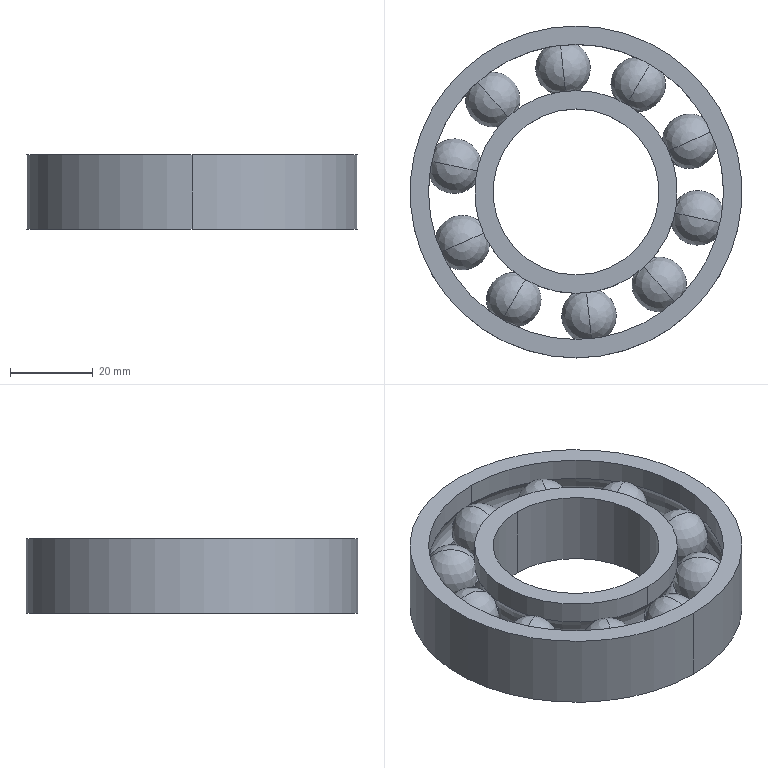Part | NX | features BREP 12 | 12 solids | 40 faces | box 80 x 80 x 18 mm | volume 40475 mm3 | sphere 20 | cylinder 12 | plane 4 | torus 4 | commonest cylinder face diameters 48.889 x4 71.111 x4 40 x2 80 x2
STEP:
#1=CARTESIAN_POINT('',(-27.406,-12.202,-6.667));
#2=VERTEX_POINT('',#1);
#3=CARTESIAN_POINT('',(-27.406,-12.202,6.667));
#4=VERTEX_POINT('',#3);
#5=CARTESIAN_POINT('',(-27.406,-12.202,0.));
#6=DIRECTION('',(0.4067,-0.9135,0.));
#7=DIRECTION('',(0.,0.,-1.));
#8=AXIS2_PLACEMENT_3D('',#5,#6,#7);
#9=CIRCLE('',#8,6.667);
#10=EDGE_CURVE('',#2,#4,#9,.T.);
#11=ORIENTED_EDGE('',*,*,#10,.F.);
#12=CARTESIAN_POINT('',(-27.406,-12.202,0.));
#13=DIRECTION('',(-0.4067,0.9135,0.));
#14=DIRECTION('',(0.,0.,-1.));
#15=AXIS2_PLACEMENT_3D('',#12,#13,#14);
#16=CIRCLE('',#15,6.667);
#17=EDGE_CURVE('',#2,#4,#16,.T.);
#18=ORIENTED_EDGE('',*,*,#17,.T.);
#19=EDGE_LOOP('',(#11,#18));
#20=FACE_BOUND('',#19,.T.);
#21=CARTESIAN_POINT('',(-27.406,-12.202,0.));
#22=DIRECTION('',(0.,0.,-1.));
#23=DIRECTION('',(-0.9135,-0.4067,0.));
#24=AXIS2_PLACEMENT_3D('',#21,#22,#23);
#25=SPHERICAL_SURFACE('',#24,6.667);
#26=ADVANCED_FACE('',(#20),#25,.T.);
#27=ORIENTED_EDGE('',*,*,#10,.T.);
#28=ORIENTED_EDGE('',*,*,#17,.F.);
#29=EDGE_LOOP('',(#27,#28));
#30=FACE_BOUND('',#29,.T.);
#31=CARTESIAN_POINT('',(-27.406,-12.202,0.));
#32=DIRECTION('',(0.,0.,-1.));
#33=DIRECTION('',(-0.9135,-0.4067,0.));
#34=AXIS2_PLACEMENT_3D('',#31,#32,#33);
#35=SPHERICAL_SURFACE('',#34,6.667);
#36=ADVANCED_FACE('',(#30),#35,.T.);
#37=CLOSED_SHELL('',(#26,#36));
#38=MANIFOLD_SOLID_BREP('',#37);
#39=CARTESIAN_POINT('',(0.,40.,-9.));
#40=VERTEX_POINT('',#39);
#41=CARTESIAN_POINT('',(0.,-40.,-9.));
#42=VERTEX_POINT('',#41);
#43=CARTESIAN_POINT('',(0.,0.,-9.));
#44=DIRECTION('',(0.,0.,1.));
#45=DIRECTION('',(0.,1.,0.));
#46=AXIS2_PLACEMENT_3D('',#43,#44,#45);
#47=CIRCLE('',#46,40.);
#48=EDGE_CURVE('',#40,#42,#47,.T.);
#49=ORIENTED_EDGE('',*,*,#48,.T.);
#50=CARTESIAN_POINT('',(0.,-40.,9.));
#51=VERTEX_POINT('',#50);
#52=CARTESIAN_POINT('',(0.,-40.,-9.));
#53=DIRECTION('',(0.,0.,1.));
#54=VECTOR('',#53,1000.);
#55=LINE('',#52,#54);
#56=EDGE_CURVE('',#42,#51,#55,.T.);
#57=ORIENTED_EDGE('',*,*,#56,.T.);
#58=CARTESIAN_POINT('',(0.,40.,9.));
#59=VERTEX_POINT('',#58);
#60=CARTESIAN_POINT('',(0.,0.,9.));
#61=DIRECTION('',(0.,0.,1.));
#62=DIRECTION('',(0.,1.,0.));
#63=AXIS2_PLACEMENT_3D('',#60,#61,#62);
#64=CIRCLE('',#63,40.);
#65=EDGE_CURVE('',#59,#51,#64,.T.);
#66=ORIENTED_EDGE('',*,*,#65,.F.);
#67=CARTESIAN_POINT('',(0.,40.,-9.));
#68=DIRECTION('',(0.,0.,1.));
#69=VECTOR('',#68,1000.);
#70=LINE('',#67,#69);
#71=EDGE_CURVE('',#40,#59,#70,.T.);
#72=ORIENTED_EDGE('',*,*,#71,.F.);
#73=EDGE_LOOP('',(#49,#57,#66,#72));
#74=FACE_BOUND('',#73,.T.);
#75=CARTESIAN_POINT('',(0.,0.,9.9));
#76=DIRECTION('',(0.,0.,-1.));
#77=DIRECTION('',(0.,1.,0.));
#78=AXIS2_PLACEMENT_3D('',#75,#76,#77);
#79=CYLINDRICAL_SURFACE('',#78,40.);
#80=ADVANCED_FACE('',(#74),#79,.T.);
#81=CARTESIAN_POINT('',(0.,0.,9.));
#82=DIRECTION('',(0.,0.,-1.));
#83=DIRECTION('',(0.,1.,0.));
#84=AXIS2_PLACEMENT_3D('',#81,#82,#83);
#85=CIRCLE('',#84,40.);
#86=EDGE_CURVE('',#59,#51,#85,.T.);
#87=ORIENTED_EDGE('',*,*,#86,.T.);
#88=ORIENTED_EDGE('',*,*,#56,.F.);
#89=CARTESIAN_POINT('',(0.,0.,-9.));
#90=DIRECTION('',(0.,0.,-1.));
#91=DIRECTION('',(0.,1.,0.));
#92=AXIS2_PLACEMENT_3D('',#89,#90,#91);
#93=CIRCLE('',#92,40.);
#94=EDGE_CURVE('',#40,#42,#93,.T.);
#95=ORIENTED_EDGE('',*,*,#94,.F.);
#96=ORIENTED_EDGE('',*,*,#71,.T.);
#97=EDGE_LOOP('',(#87,#88,#95,#96));
#98=FACE_BOUND('',#97,.T.);
#99=CARTESIAN_POINT('',(0.,0.,9.9));
#100=DIRECTION('',(0.,0.,-1.));
#101=DIRECTION('',(0.,1.,0.));
#102=AXIS2_PLACEMENT_3D('',#99,#100,#101);
#103=CYLINDRICAL_SURFACE('',#102,40.);
#104=ADVANCED_FACE('',(#98),#103,.T.);
#105=ORIENTED_EDGE('',*,*,#48,.F.);
#106=ORIENTED_EDGE('',*,*,#94,.T.);
#107=EDGE_LOOP('',(#105,#106));
#108=FACE_BOUND('',#107,.T.);
#109=CARTESIAN_POINT('',(0.,35.556,-9.));
#110=VERTEX_POINT('',#109);
#111=CARTESIAN_POINT('',(0.,-35.556,-9.));
#112=VERTEX_POINT('',#111);
#113=CARTESIAN_POINT('',(0.,0.,-9.));
#114=DIRECTION('',(0.,0.,-1.));
#115=DIRECTION('',(0.,1.,0.));
#116=AXIS2_PLACEMENT_3D('',#113,#114,#115);
#117=CIRCLE('',#116,35.556);
#118=EDGE_CURVE('',#110,#112,#117,.T.);
#119=ORIENTED_EDGE('',*,*,#118,.F.);
#120=CARTESIAN_POINT('',(0.,0.,-9.));
#121=DIRECTION('',(0.,0.,1.));
#122=DIRECTION('',(0.,1.,0.));
#123=AXIS2_PLACEMENT_3D('',#120,#121,#122);
#124=CIRCLE('',#123,35.556);
#125=EDGE_CURVE('',#110,#112,#124,.T.);
#126=ORIENTED_EDGE('',*,*,#125,.T.);
#127=EDGE_LOOP('',(#119,#126));
#128=FACE_BOUND('',#127,.T.);
#129=CARTESIAN_POINT('',(0.,0.,-9.));
#130=DIRECTION('',(0.,0.,-1.));
#131=DIRECTION('',(0.,1.,0.));
#132=AXIS2_PLACEMENT_3D('',#129,#130,#131);
#133=PLANE('',#132);
#134=ADVANCED_FACE('',(#108,#128),#133,.T.);
#135=CARTESIAN_POINT('',(0.,35.556,-3.685));
#136=VERTEX_POINT('',#135);
#137=CARTESIAN_POINT('',(0.,-35.556,-3.685));
#138=VERTEX_POINT('',#137);
#139=CARTESIAN_POINT('',(0.,0.,-3.685));
#140=DIRECTION('',(0.,0.,1.));
#141=DIRECTION('',(0.,1.,0.));
#142=AXIS2_PLACEMENT_3D('',#139,#140,#141);
#143=CIRCLE('',#142,35.556);
#144=EDGE_CURVE('',#136,#138,#143,.T.);
#145=ORIENTED_EDGE('',*,*,#144,.T.);
#146=CARTESIAN_POINT('',(0.,-35.556,-3.685));
#147=DIRECTION('',(0.,0.,-1.));
#148=VECTOR('',#147,1000.);
#149=LINE('',#146,#148);
#150=EDGE_CURVE('',#138,#112,#149,.T.);
#151=ORIENTED_EDGE('',*,*,#150,.T.);
#152=ORIENTED_EDGE('',*,*,#125,.F.);
#153=CARTESIAN_POINT('',(0.,35.556,-3.685));
#154=DIRECTION('',(0.,0.,-1.));
#155=VECTOR('',#154,1000.);
#156=LINE('',#153,#155);
#157=EDGE_CURVE('',#136,#110,#156,.T.);
#158=ORIENTED_EDGE('',*,*,#157,.F.);
#159=EDGE_LOOP('',(#145,#151,#152,#158));
#160=FACE_BOUND('',#159,.T.);
#161=CARTESIAN_POINT('',(0.,0.,9.9));
#162=DIRECTION('',(0.,0.,-1.));
#163=DIRECTION('',(0.,1.,0.));
#164=AXIS2_PLACEMENT_3D('',#161,#162,#163);
#165=CYLINDRICAL_SURFACE('',#164,35.556);
#166=ADVANCED_FACE('',(#160),#165,.F.);
#167=ORIENTED_EDGE('',*,*,#118,.T.);
#168=ORIENTED_EDGE('',*,*,#150,.F.);
#169=CARTESIAN_POINT('',(0.,0.,-3.685));
#170=DIRECTION('',(0.,0.,-1.));
#171=DIRECTION('',(0.,1.,0.));
#172=AXIS2_PLACEMENT_3D('',#169,#170,#171);
#173=CIRCLE('',#172,35.556);
#174=EDGE_CURVE('',#136,#138,#173,.T.);
#175=ORIENTED_EDGE('',*,*,#174,.F.);
#176=ORIENTED_EDGE('',*,*,#157,.T.);
#177=EDGE_LOOP('',(#167,#168,#175,#176));
#178=FACE_BOUND('',#177,.T.);
#179=CARTESIAN_POINT('',(0.,0.,9.9));
#180=DIRECTION('',(0.,0.,-1.));
#181=DIRECTION('',(0.,1.,0.));
#182=AXIS2_PLACEMENT_3D('',#179,#180,#181);
#183=CYLINDRICAL_SURFACE('',#182,35.556);
#184=ADVANCED_FACE('',(#178),#183,.F.);
#185=ORIENTED_EDGE('',*,*,#174,.T.);
#186=CARTESIAN_POINT('',(0.,-35.556,3.685));
#187=VERTEX_POINT('',#186);
#188=CARTESIAN_POINT('',(0.,-30.,0.));
#189=DIRECTION('',(1.,0.,0.));
#190=DIRECTION('',(0.,-0.8333,0.5528));
#191=AXIS2_PLACEMENT_3D('',#188,#189,#190);
#192=CIRCLE('',#191,6.667);
#193=EDGE_CURVE('',#138,#187,#192,.F.);
#194=ORIENTED_EDGE('',*,*,#193,.T.);
#195=CARTESIAN_POINT('',(0.,35.556,3.685));
#196=VERTEX_POINT('',#195);
#197=CARTESIAN_POINT('',(0.,0.,3.685));
#198=DIRECTION('',(0.,0.,-1.));
#199=DIRECTION('',(0.,1.,0.));
#200=AXIS2_PLACEMENT_3D('',#197,#198,#199);
#201=CIRCLE('',#200,35.556);
#202=EDGE_CURVE('',#196,#187,#201,.T.);
#203=ORIENTED_EDGE('',*,*,#202,.F.);
#204=CARTESIAN_POINT('',(0.,30.,0.));
#205=DIRECTION('',(-1.,0.,0.));
#206=DIRECTION('',(0.,0.8333,0.5528));
#207=AXIS2_PLACEMENT_3D('',#204,#205,#206);
#208=CIRCLE('',#207,6.667);
#209=EDGE_CURVE('',#136,#196,#208,.F.);
#210=ORIENTED_EDGE('',*,*,#209,.F.);
#211=EDGE_LOOP('',(#185,#194,#203,#210));
#212=FACE_BOUND('',#211,.T.);
#213=CARTESIAN_POINT('',(0.,0.,0.));
#214=DIRECTION('',(0.,0.,-1.));
#215=DIRECTION('',(0.,1.,0.));
#216=AXIS2_PLACEMENT_3D('',#213,#214,#215);
#217=TOROIDAL_SURFACE('',#216,30.,6.667);
#218=ADVANCED_FACE('',(#212),#217,.F.);
#219=CARTESIAN_POINT('',(0.,0.,3.685));
#220=DIRECTION('',(0.,0.,1.));
#221=DIRECTION('',(0.,1.,0.));
#222=AXIS2_PLACEMENT_3D('',#219,#220,#221);
#223=CIRCLE('',#222,35.556);
#224=EDGE_CURVE('',#196,#187,#223,.T.);
#225=ORIENTED_EDGE('',*,*,#224,.T.);
#226=ORIENTED_EDGE('',*,*,#193,.F.);
#227=ORIENTED_EDGE('',*,*,#144,.F.);
#228=ORIENTED_EDGE('',*,*,#209,.T.);
#229=EDGE_LOOP('',(#225,#226,#227,#228));
#230=FACE_BOUND('',#229,.T.);
#231=CARTESIAN_POINT('',(0.,0.,0.));
#232=DIRECTION('',(0.,0.,-1.));
#233=DIRECTION('',(0.,1.,0.));
#234=AXIS2_PLACEMENT_3D('',#231,#232,#233);
#235=TOROIDAL_SURFACE('',#234,30.,6.667);
#236=ADVANCED_FACE('',(#230),#235,.F.);
#237=CARTESIAN_POINT('',(0.,35.556,9.));
#238=VERTEX_POINT('',#237);
#239=CARTESIAN_POINT('',(0.,-35.556,9.));
#240=VERTEX_POINT('',#239);
#241=CARTESIAN_POINT('',(0.,0.,9.));
#242=DIRECTION('',(0.,0.,1.));
#243=DIRECTION('',(0.,1.,0.));
#244=AXIS2_PLACEMENT_3D('',#241,#242,#243);
#245=CIRCLE('',#244,35.556);
#246=EDGE_CURVE('',#238,#240,#245,.T.);
#247=ORIENTED_EDGE('',*,*,#246,.T.);
#248=CARTESIAN_POINT('',(0.,-35.556,9.));
#249=DIRECTION('',(0.,0.,-1.));
#250=VECTOR('',#249,1000.);
#251=LINE('',#248,#250);
#252=EDGE_CURVE('',#240,#187,#251,.T.);
#253=ORIENTED_EDGE('',*,*,#252,.T.);
#254=ORIENTED_EDGE('',*,*,#224,.F.);
#255=CARTESIAN_POINT('',(0.,35.556,9.));
#256=DIRECTION('',(0.,0.,-1.));
#257=VECTOR('',#256,1000.);
#258=LINE('',#255,#257);
#259=EDGE_CURVE('',#238,#196,#258,.T.);
#260=ORIENTED_EDGE('',*,*,#259,.F.);
#261=EDGE_LOOP('',(#247,#253,#254,#260));
#262=FACE_BOUND('',#261,.T.);
#263=CARTESIAN_POINT('',(0.,0.,9.9));
#264=DIRECTION('',(0.,0.,-1.));
#265=DIRECTION('',(0.,1.,0.));
#266=AXIS2_PLACEMENT_3D('',#263,#264,#265);
#267=CYLINDRICAL_SURFACE('',#266,35.556);
#268=ADVANCED_FACE('',(#262),#267,.F.);
#269=ORIENTED_EDGE('',*,*,#202,.T.);
#270=ORIENTED_EDGE('',*,*,#252,.F.);
#271=CARTESIAN_POINT('',(0.,0.,9.));
#272=DIRECTION('',(0.,0.,-1.));
#273=DIRECTION('',(0.,1.,0.));
#274=AXIS2_PLACEMENT_3D('',#271,#272,#273);
#275=CIRCLE('',#274,35.556);
#276=EDGE_CURVE('',#238,#240,#275,.T.);
#277=ORIENTED_EDGE('',*,*,#276,.F.);
#278=ORIENTED_EDGE('',*,*,#259,.T.);
#279=EDGE_LOOP('',(#269,#270,#277,#278));
#280=FACE_BOUND('',#279,.T.);
#281=CARTESIAN_POINT('',(0.,0.,9.9));
#282=DIRECTION('',(0.,0.,-1.));
#283=DIRECTION('',(0.,1.,0.));
#284=AXIS2_PLACEMENT_3D('',#281,#282,#283);
#285=CYLINDRICAL_SURFACE('',#284,35.556);
#286=ADVANCED_FACE('',(#280),#285,.F.);
#287=ORIENTED_EDGE('',*,*,#86,.F.);
#288=ORIENTED_EDGE('',*,*,#65,.T.);
#289=EDGE_LOOP('',(#287,#288));
#290=FACE_BOUND('',#289,.T.);
#291=ORIENTED_EDGE('',*,*,#246,.F.);
#292=ORIENTED_EDGE('',*,*,#276,.T.);
#293=EDGE_LOOP('',(#291,#292));
#294=FACE_BOUND('',#293,.T.);
#295=CARTESIAN_POINT('',(0.,0.,9.));
#296=DIRECTION('',(0.,0.,-1.));
#297=DIRECTION('',(0.,1.,0.));
#298=AXIS2_PLACEMENT_3D('',#295,#296,#297);
#299=PLANE('',#298);
#300=ADVANCED_FACE('',(#290,#294),#299,.F.);
#301=CLOSED_SHELL('',(#80,#104,#134,#166,#184,#218,#236,#268,#286,#300));
#302=MANIFOLD_SOLID_BREP('',#301);
#303=CARTESIAN_POINT('',(20.074,-22.294,6.667));
#304=VERTEX_POINT('',#303);
#305=CARTESIAN_POINT('',(20.074,-22.294,-6.667));
#306=VERTEX_POINT('',#305);
#307=CARTESIAN_POINT('',(20.074,-22.294,0.));
#308=DIRECTION('',(0.7431,0.6691,0.));
#309=DIRECTION('',(0.,0.,-1.));
#310=AXIS2_PLACEMENT_3D('',#307,#308,#309);
#311=CIRCLE('',#310,6.667);
#312=EDGE_CURVE('',#304,#306,#311,.F.);
#313=ORIENTED_EDGE('',*,*,#312,.T.);
#314=CARTESIAN_POINT('',(20.074,-22.294,0.));
#315=DIRECTION('',(-0.7431,-0.6691,0.));
#316=DIRECTION('',(0.,0.,-1.));
#317=AXIS2_PLACEMENT_3D('',#314,#315,#316);
#318=CIRCLE('',#317,6.667);
#319=EDGE_CURVE('',#304,#306,#318,.F.);
#320=ORIENTED_EDGE('',*,*,#319,.F.);
#321=EDGE_LOOP('',(#313,#320));
#322=FACE_BOUND('',#321,.T.);
#323=CARTESIAN_POINT('',(20.074,-22.294,0.));
#324=DIRECTION('',(0.,0.,-1.));
#325=DIRECTION('',(0.6691,-0.7431,0.));
#326=AXIS2_PLACEMENT_3D('',#323,#324,#325);
#327=SPHERICAL_SURFACE('',#326,6.667);
#328=ADVANCED_FACE('',(#322),#327,.T.);
#329=ORIENTED_EDGE('',*,*,#312,.F.);
#330=ORIENTED_EDGE('',*,*,#319,.T.);
#331=EDGE_LOOP('',(#329,#330));
#332=FACE_BOUND('',#331,.T.);
#333=CARTESIAN_POINT('',(20.074,-22.294,0.));
#334=DIRECTION('',(0.,0.,-1.));
#335=DIRECTION('',(0.6691,-0.7431,0.));
#336=AXIS2_PLACEMENT_3D('',#333,#334,#335);
#337=SPHERICAL_SURFACE('',#336,6.667);
#338=ADVANCED_FACE('',(#332),#337,.T.);
#339=CLOSED_SHELL('',(#328,#338));
#340=MANIFOLD_SOLID_BREP('',#339);
#341=CARTESIAN_POINT('',(-20.074,22.294,-6.667));
#342=VERTEX_POINT('',#341);
#343=CARTESIAN_POINT('',(-20.074,22.294,6.667));
#344=VERTEX_POINT('',#343);
#345=CARTESIAN_POINT('',(-20.074,22.294,0.));
#346=DIRECTION('',(-0.7431,-0.6691,0.));
#347=DIRECTION('',(0.,0.,-1.));
#348=AXIS2_PLACEMENT_3D('',#345,#346,#347);
#349=CIRCLE('',#348,6.667);
#350=EDGE_CURVE('',#342,#344,#349,.T.);
#351=ORIENTED_EDGE('',*,*,#350,.F.);
#352=CARTESIAN_POINT('',(-20.074,22.294,0.));
#353=DIRECTION('',(0.7431,0.6691,0.));
#354=DIRECTION('',(0.,0.,-1.));
#355=AXIS2_PLACEMENT_3D('',#352,#353,#354);
#356=CIRCLE('',#355,6.667);
#357=EDGE_CURVE('',#342,#344,#356,.T.);
#358=ORIENTED_EDGE('',*,*,#357,.T.);
#359=EDGE_LOOP('',(#351,#358));
#360=FACE_BOUND('',#359,.T.);
#361=CARTESIAN_POINT('',(-20.074,22.294,0.));
#362=DIRECTION('',(0.,0.,-1.));
#363=DIRECTION('',(-0.6691,0.7431,0.));
#364=AXIS2_PLACEMENT_3D('',#361,#362,#363);
#365=SPHERICAL_SURFACE('',#364,6.667);
#366=ADVANCED_FACE('',(#360),#365,.T.);
#367=ORIENTED_EDGE('',*,*,#350,.T.);
#368=ORIENTED_EDGE('',*,*,#357,.F.);
#369=EDGE_LOOP('',(#367,#368));
#370=FACE_BOUND('',#369,.T.);
#371=CARTESIAN_POINT('',(-20.074,22.294,0.));
#372=DIRECTION('',(0.,0.,-1.));
#373=DIRECTION('',(-0.6691,0.7431,0.));
#374=AXIS2_PLACEMENT_3D('',#371,#372,#373);
#375=SPHERICAL_SURFACE('',#374,6.667);
#376=ADVANCED_FACE('',(#370),#375,.T.);
#377=CLOSED_SHELL('',(#366,#376));
#378=MANIFOLD_SOLID_BREP('',#377);
#379=CARTESIAN_POINT('',(-15.,-25.981,-6.667));
#380=VERTEX_POINT('',#379);
#381=CARTESIAN_POINT('',(-15.,-25.981,6.667));
#382=VERTEX_POINT('',#381);
#383=CARTESIAN_POINT('',(-15.,-25.981,0.));
#384=DIRECTION('',(0.866,-0.5,0.));
#385=DIRECTION('',(0.,0.,-1.));
#386=AXIS2_PLACEMENT_3D('',#383,#384,#385);
#387=CIRCLE('',#386,6.667);
#388=EDGE_CURVE('',#380,#382,#387,.T.);
#389=ORIENTED_EDGE('',*,*,#388,.F.);
#390=CARTESIAN_POINT('',(-15.,-25.981,0.));
#391=DIRECTION('',(-0.866,0.5,0.));
#392=DIRECTION('',(0.,0.,-1.));
#393=AXIS2_PLACEMENT_3D('',#390,#391,#392);
#394=CIRCLE('',#393,6.667);
#395=EDGE_CURVE('',#380,#382,#394,.T.);
#396=ORIENTED_EDGE('',*,*,#395,.T.);
#397=EDGE_LOOP('',(#389,#396));
#398=FACE_BOUND('',#397,.T.);
#399=CARTESIAN_POINT('',(-15.,-25.981,0.));
#400=DIRECTION('',(0.,0.,-1.));
#401=DIRECTION('',(-0.5,-0.866,0.));
#402=AXIS2_PLACEMENT_3D('',#399,#400,#401);
#403=SPHERICAL_SURFACE('',#402,6.667);
#404=ADVANCED_FACE('',(#398),#403,.T.);
#405=ORIENTED_EDGE('',*,*,#388,.T.);
#406=ORIENTED_EDGE('',*,*,#395,.F.);
#407=EDGE_LOOP('',(#405,#406));
#408=FACE_BOUND('',#407,.T.);
#409=CARTESIAN_POINT('',(-15.,-25.981,0.));
#410=DIRECTION('',(0.,0.,-1.));
#411=DIRECTION('',(-0.5,-0.866,0.));
#412=AXIS2_PLACEMENT_3D('',#409,#410,#411);
#413=SPHERICAL_SURFACE('',#412,6.667);
#414=ADVANCED_FACE('',(#408),#413,.T.);
#415=CLOSED_SHELL('',(#404,#414));
#416=MANIFOLD_SOLID_BREP('',#415);
#417=CARTESIAN_POINT('',(-3.136,29.836,-6.667));
#418=VERTEX_POINT('',#417);
#419=CARTESIAN_POINT('',(-3.136,29.836,6.667));
#420=VERTEX_POINT('',#419);
#421=CARTESIAN_POINT('',(-3.136,29.836,0.));
#422=DIRECTION('',(-0.9945,-0.1045,0.));
#423=DIRECTION('',(0.,0.,-1.));
#424=AXIS2_PLACEMENT_3D('',#421,#422,#423);
#425=CIRCLE('',#424,6.667);
#426=EDGE_CURVE('',#418,#420,#425,.T.);
#427=ORIENTED_EDGE('',*,*,#426,.F.);
#428=CARTESIAN_POINT('',(-3.136,29.836,0.));
#429=DIRECTION('',(0.9945,0.1045,0.));
#430=DIRECTION('',(0.,0.,-1.));
#431=AXIS2_PLACEMENT_3D('',#428,#429,#430);
#432=CIRCLE('',#431,6.667);
#433=EDGE_CURVE('',#418,#420,#432,.T.);
#434=ORIENTED_EDGE('',*,*,#433,.T.);
#435=EDGE_LOOP('',(#427,#434));
#436=FACE_BOUND('',#435,.T.);
#437=CARTESIAN_POINT('',(-3.136,29.836,0.));
#438=DIRECTION('',(0.,0.,-1.));
#439=DIRECTION('',(-0.1045,0.9945,0.));
#440=AXIS2_PLACEMENT_3D('',#437,#438,#439);
#441=SPHERICAL_SURFACE('',#440,6.667);
#442=ADVANCED_FACE('',(#436),#441,.T.);
#443=ORIENTED_EDGE('',*,*,#426,.T.);
#444=ORIENTED_EDGE('',*,*,#433,.F.);
#445=EDGE_LOOP('',(#443,#444));
#446=FACE_BOUND('',#445,.T.);
#447=CARTESIAN_POINT('',(-3.136,29.836,0.));
#448=DIRECTION('',(0.,0.,-1.));
#449=DIRECTION('',(-0.1045,0.9945,0.));
#450=AXIS2_PLACEMENT_3D('',#447,#448,#449);
#451=SPHERICAL_SURFACE('',#450,6.667);
#452=ADVANCED_FACE('',(#446),#451,.T.);
#453=CLOSED_SHELL('',(#442,#452));
#454=MANIFOLD_SOLID_BREP('',#453);
#455=CARTESIAN_POINT('',(-29.344,6.237,-6.667));
#456=VERTEX_POINT('',#455);
#457=CARTESIAN_POINT('',(-29.344,6.237,6.667));
#458=VERTEX_POINT('',#457);
#459=CARTESIAN_POINT('',(-29.344,6.237,0.));
#460=DIRECTION('',(-0.2079,-0.9781,0.));
#461=DIRECTION('',(0.,0.,-1.));
#462=AXIS2_PLACEMENT_3D('',#459,#460,#461);
#463=CIRCLE('',#462,6.667);
#464=EDGE_CURVE('',#456,#458,#463,.T.);
#465=ORIENTED_EDGE('',*,*,#464,.F.);
#466=CARTESIAN_POINT('',(-29.344,6.237,0.));
#467=DIRECTION('',(0.2079,0.9781,0.));
#468=DIRECTION('',(0.,0.,-1.));
#469=AXIS2_PLACEMENT_3D('',#466,#467,#468);
#470=CIRCLE('',#469,6.667);
#471=EDGE_CURVE('',#456,#458,#470,.T.);
#472=ORIENTED_EDGE('',*,*,#471,.T.);
#473=EDGE_LOOP('',(#465,#472));
#474=FACE_BOUND('',#473,.T.);
#475=CARTESIAN_POINT('',(-29.344,6.237,0.));
#476=DIRECTION('',(0.,0.,-1.));
#477=DIRECTION('',(-0.9781,0.2079,0.));
#478=AXIS2_PLACEMENT_3D('',#475,#476,#477);
#479=SPHERICAL_SURFACE('',#478,6.667);
#480=ADVANCED_FACE('',(#474),#479,.T.);
#481=ORIENTED_EDGE('',*,*,#464,.T.);
#482=ORIENTED_EDGE('',*,*,#471,.F.);
#483=EDGE_LOOP('',(#481,#482));
#484=FACE_BOUND('',#483,.T.);
#485=CARTESIAN_POINT('',(-29.344,6.237,0.));
#486=DIRECTION('',(0.,0.,-1.));
#487=DIRECTION('',(-0.9781,0.2079,0.));
#488=AXIS2_PLACEMENT_3D('',#485,#486,#487);
#489=SPHERICAL_SURFACE('',#488,6.667);
#490=ADVANCED_FACE('',(#484),#489,.T.);
#491=CLOSED_SHELL('',(#480,#490));
#492=MANIFOLD_SOLID_BREP('',#491);
#493=CARTESIAN_POINT('',(27.406,12.202,6.667));
#494=VERTEX_POINT('',#493);
#495=CARTESIAN_POINT('',(27.406,12.202,-6.667));
#496=VERTEX_POINT('',#495);
#497=CARTESIAN_POINT('',(27.406,12.202,0.));
#498=DIRECTION('',(-0.4067,0.9135,0.));
#499=DIRECTION('',(0.,0.,-1.));
#500=AXIS2_PLACEMENT_3D('',#497,#498,#499);
#501=CIRCLE('',#500,6.667);
#502=EDGE_CURVE('',#494,#496,#501,.F.);
#503=ORIENTED_EDGE('',*,*,#502,.T.);
#504=CARTESIAN_POINT('',(27.406,12.202,0.));
#505=DIRECTION('',(0.4067,-0.9135,0.));
#506=DIRECTION('',(0.,0.,-1.));
#507=AXIS2_PLACEMENT_3D('',#504,#505,#506);
#508=CIRCLE('',#507,6.667);
#509=EDGE_CURVE('',#494,#496,#508,.F.);
#510=ORIENTED_EDGE('',*,*,#509,.F.);
#511=EDGE_LOOP('',(#503,#510));
#512=FACE_BOUND('',#511,.T.);
#513=CARTESIAN_POINT('',(27.406,12.202,0.));
#514=DIRECTION('',(0.,0.,-1.));
#515=DIRECTION('',(0.9135,0.4067,0.));
#516=AXIS2_PLACEMENT_3D('',#513,#514,#515);
#517=SPHERICAL_SURFACE('',#516,6.667);
#518=ADVANCED_FACE('',(#512),#517,.T.);
#519=ORIENTED_EDGE('',*,*,#502,.F.);
#520=ORIENTED_EDGE('',*,*,#509,.T.);
#521=EDGE_LOOP('',(#519,#520));
#522=FACE_BOUND('',#521,.T.);
#523=CARTESIAN_POINT('',(27.406,12.202,0.));
#524=DIRECTION('',(0.,0.,-1.));
#525=DIRECTION('',(0.9135,0.4067,0.));
#526=AXIS2_PLACEMENT_3D('',#523,#524,#525);
#527=SPHERICAL_SURFACE('',#526,6.667);
#528=ADVANCED_FACE('',(#522),#527,.T.);
#529=CLOSED_SHELL('',(#518,#528));
#530=MANIFOLD_SOLID_BREP('',#529);
#531=CARTESIAN_POINT('',(3.136,-29.836,6.667));
#532=VERTEX_POINT('',#531);
#533=CARTESIAN_POINT('',(3.136,-29.836,-6.667));
#534=VERTEX_POINT('',#533);
#535=CARTESIAN_POINT('',(3.136,-29.836,0.));
#536=DIRECTION('',(0.9945,0.1045,0.));
#537=DIRECTION('',(0.,0.,-1.));
#538=AXIS2_PLACEMENT_3D('',#535,#536,#537);
#539=CIRCLE('',#538,6.667);
#540=EDGE_CURVE('',#532,#534,#539,.F.);
#541=ORIENTED_EDGE('',*,*,#540,.T.);
#542=CARTESIAN_POINT('',(3.136,-29.836,0.));
#543=DIRECTION('',(-0.9945,-0.1045,0.));
#544=DIRECTION('',(0.,0.,-1.));
#545=AXIS2_PLACEMENT_3D('',#542,#543,#544);
#546=CIRCLE('',#545,6.667);
#547=EDGE_CURVE('',#532,#534,#546,.F.);
#548=ORIENTED_EDGE('',*,*,#547,.F.);
#549=EDGE_LOOP('',(#541,#548));
#550=FACE_BOUND('',#549,.T.);
#551=CARTESIAN_POINT('',(3.136,-29.836,0.));
#552=DIRECTION('',(0.,0.,-1.));
#553=DIRECTION('',(0.1045,-0.9945,0.));
#554=AXIS2_PLACEMENT_3D('',#551,#552,#553);
#555=SPHERICAL_SURFACE('',#554,6.667);
#556=ADVANCED_FACE('',(#550),#555,.T.);
#557=ORIENTED_EDGE('',*,*,#540,.F.);
#558=ORIENTED_EDGE('',*,*,#547,.T.);
#559=EDGE_LOOP('',(#557,#558));
#560=FACE_BOUND('',#559,.T.);
#561=CARTESIAN_POINT('',(3.136,-29.836,0.));
#562=DIRECTION('',(0.,0.,-1.));
#563=DIRECTION('',(0.1045,-0.9945,0.));
#564=AXIS2_PLACEMENT_3D('',#561,#562,#563);
#565=SPHERICAL_SURFACE('',#564,6.667);
#566=ADVANCED_FACE('',(#560),#565,.T.);
#567=CLOSED_SHELL('',(#556,#566));
#568=MANIFOLD_SOLID_BREP('',#567);
#569=CARTESIAN_POINT('',(15.,25.981,6.667));
#570=VERTEX_POINT('',#569);
#571=CARTESIAN_POINT('',(15.,25.981,-6.667));
#572=VERTEX_POINT('',#571);
#573=CARTESIAN_POINT('',(15.,25.981,0.));
#574=DIRECTION('',(-0.866,0.5,0.));
#575=DIRECTION('',(0.,0.,-1.));
#576=AXIS2_PLACEMENT_3D('',#573,#574,#575);
#577=CIRCLE('',#576,6.667);
#578=EDGE_CURVE('',#570,#572,#577,.F.);
#579=ORIENTED_EDGE('',*,*,#578,.T.);
#580=CARTESIAN_POINT('',(15.,25.981,0.));
#581=DIRECTION('',(0.866,-0.5,0.));
#582=DIRECTION('',(0.,0.,-1.));
#583=AXIS2_PLACEMENT_3D('',#580,#581,#582);
#584=CIRCLE('',#583,6.667);
#585=EDGE_CURVE('',#570,#572,#584,.F.);
#586=ORIENTED_EDGE('',*,*,#585,.F.);
#587=EDGE_LOOP('',(#579,#586));
#588=FACE_BOUND('',#587,.T.);
#589=CARTESIAN_POINT('',(15.,25.981,0.));
#590=DIRECTION('',(0.,0.,-1.));
#591=DIRECTION('',(0.5,0.866,0.));
#592=AXIS2_PLACEMENT_3D('',#589,#590,#591);
#593=SPHERICAL_SURFACE('',#592,6.667);
#594=ADVANCED_FACE('',(#588),#593,.T.);
#595=ORIENTED_EDGE('',*,*,#578,.F.);
#596=ORIENTED_EDGE('',*,*,#585,.T.);
#597=EDGE_LOOP('',(#595,#596));
#598=FACE_BOUND('',#597,.T.);
#599=CARTESIAN_POINT('',(15.,25.981,0.));
#600=DIRECTION('',(0.,0.,-1.));
#601=DIRECTION('',(0.5,0.866,0.));
#602=AXIS2_PLACEMENT_3D('',#599,#600,#601);
#603=SPHERICAL_SURFACE('',#602,6.667);
#604=ADVANCED_FACE('',(#598),#603,.T.);
#605=CLOSED_SHELL('',(#594,#604));
#606=MANIFOLD_SOLID_BREP('',#605);
#607=CARTESIAN_POINT('',(29.344,-6.237,6.667));
#608=VERTEX_POINT('',#607);
#609=CARTESIAN_POINT('',(29.344,-6.237,-6.667));
#610=VERTEX_POINT('',#609);
#611=CARTESIAN_POINT('',(29.344,-6.237,0.));
#612=DIRECTION('',(0.2079,0.9781,0.));
#613=DIRECTION('',(0.,0.,-1.));
#614=AXIS2_PLACEMENT_3D('',#611,#612,#613);
#615=CIRCLE('',#614,6.667);
#616=EDGE_CURVE('',#608,#610,#615,.F.);
#617=ORIENTED_EDGE('',*,*,#616,.T.);
#618=CARTESIAN_POINT('',(29.344,-6.237,0.));
#619=DIRECTION('',(-0.2079,-0.9781,0.));
#620=DIRECTION('',(0.,0.,-1.));
#621=AXIS2_PLACEMENT_3D('',#618,#619,#620);
#622=CIRCLE('',#621,6.667);
#623=EDGE_CURVE('',#608,#610,#622,.F.);
#624=ORIENTED_EDGE('',*,*,#623,.F.);
#625=EDGE_LOOP('',(#617,#624));
#626=FACE_BOUND('',#625,.T.);
#627=CARTESIAN_POINT('',(29.344,-6.237,0.));
#628=DIRECTION('',(0.,0.,-1.));
#629=DIRECTION('',(0.9781,-0.2079,0.));
#630=AXIS2_PLACEMENT_3D('',#627,#628,#629);
#631=SPHERICAL_SURFACE('',#630,6.667);
#632=ADVANCED_FACE('',(#626),#631,.T.);
#633=ORIENTED_EDGE('',*,*,#616,.F.);
#634=ORIENTED_EDGE('',*,*,#623,.T.);
#635=EDGE_LOOP('',(#633,#634));
#636=FACE_BOUND('',#635,.T.);
#637=CARTESIAN_POINT('',(29.344,-6.237,0.));
#638=DIRECTION('',(0.,0.,-1.));
#639=DIRECTION('',(0.9781,-0.2079,0.));
#640=AXIS2_PLACEMENT_3D('',#637,#638,#639);
#641=SPHERICAL_SURFACE('',#640,6.667);
#642=ADVANCED_FACE('',(#636),#641,.T.);
#643=CLOSED_SHELL('',(#632,#642));
#644=MANIFOLD_SOLID_BREP('',#643);
#645=CARTESIAN_POINT('',(0.,24.444,3.685));
#646=VERTEX_POINT('',#645);
#647=CARTESIAN_POINT('',(0.,-24.444,3.685));
#648=VERTEX_POINT('',#647);
#649=CARTESIAN_POINT('',(0.,0.,3.685));
#650=DIRECTION('',(0.,0.,1.));
#651=DIRECTION('',(0.,1.,0.));
#652=AXIS2_PLACEMENT_3D('',#649,#650,#651);
#653=CIRCLE('',#652,24.444);
#654=EDGE_CURVE('',#646,#648,#653,.T.);
#655=ORIENTED_EDGE('',*,*,#654,.T.);
#656=CARTESIAN_POINT('',(0.,-24.444,9.));
#657=VERTEX_POINT('',#656);
#658=CARTESIAN_POINT('',(0.,-24.444,3.685));
#659=DIRECTION('',(0.,0.,1.));
#660=VECTOR('',#659,1000.);
#661=LINE('',#658,#660);
#662=EDGE_CURVE('',#648,#657,#661,.T.);
#663=ORIENTED_EDGE('',*,*,#662,.T.);
#664=CARTESIAN_POINT('',(0.,24.444,9.));
#665=VERTEX_POINT('',#664);
#666=CARTESIAN_POINT('',(0.,0.,9.));
#667=DIRECTION('',(0.,0.,1.));
#668=DIRECTION('',(0.,1.,0.));
#669=AXIS2_PLACEMENT_3D('',#666,#667,#668);
#670=CIRCLE('',#669,24.444);
#671=EDGE_CURVE('',#665,#657,#670,.T.);
#672=ORIENTED_EDGE('',*,*,#671,.F.);
#673=CARTESIAN_POINT('',(0.,24.444,3.685));
#674=DIRECTION('',(0.,0.,1.));
#675=VECTOR('',#674,1000.);
#676=LINE('',#673,#675);
#677=EDGE_CURVE('',#646,#665,#676,.T.);
#678=ORIENTED_EDGE('',*,*,#677,.F.);
#679=EDGE_LOOP('',(#655,#663,#672,#678));
#680=FACE_BOUND('',#679,.T.);
#681=CARTESIAN_POINT('',(0.,0.,9.9));
#682=DIRECTION('',(0.,0.,-1.));
#683=DIRECTION('',(0.,1.,0.));
#684=AXIS2_PLACEMENT_3D('',#681,#682,#683);
#685=CYLINDRICAL_SURFACE('',#684,24.444);
#686=ADVANCED_FACE('',(#680),#685,.T.);
#687=CARTESIAN_POINT('',(0.,0.,9.));
#688=DIRECTION('',(0.,0.,-1.));
#689=DIRECTION('',(0.,1.,0.));
#690=AXIS2_PLACEMENT_3D('',#687,#688,#689);
#691=CIRCLE('',#690,24.444);
#692=EDGE_CURVE('',#665,#657,#691,.T.);
#693=ORIENTED_EDGE('',*,*,#692,.T.);
#694=ORIENTED_EDGE('',*,*,#662,.F.);
#695=CARTESIAN_POINT('',(0.,0.,3.685));
#696=DIRECTION('',(0.,0.,-1.));
#697=DIRECTION('',(0.,1.,0.));
#698=AXIS2_PLACEMENT_3D('',#695,#696,#697);
#699=CIRCLE('',#698,24.444);
#700=EDGE_CURVE('',#646,#648,#699,.T.);
#701=ORIENTED_EDGE('',*,*,#700,.F.);
#702=ORIENTED_EDGE('',*,*,#677,.T.);
#703=EDGE_LOOP('',(#693,#694,#701,#702));
#704=FACE_BOUND('',#703,.T.);
#705=CARTESIAN_POINT('',(0.,0.,9.9));
#706=DIRECTION('',(0.,0.,-1.));
#707=DIRECTION('',(0.,1.,0.));
#708=AXIS2_PLACEMENT_3D('',#705,#706,#707);
#709=CYLINDRICAL_SURFACE('',#708,24.444);
#710=ADVANCED_FACE('',(#704),#709,.T.);
#711=ORIENTED_EDGE('',*,*,#700,.T.);
#712=CARTESIAN_POINT('',(0.,-24.444,-3.685));
#713=VERTEX_POINT('',#712);
#714=CARTESIAN_POINT('',(0.,-30.,0.));
#715=DIRECTION('',(1.,0.,0.));
#716=DIRECTION('',(0.,0.8333,-0.5528));
#717=AXIS2_PLACEMENT_3D('',#714,#715,#716);
#718=CIRCLE('',#717,6.667);
#719=EDGE_CURVE('',#648,#713,#718,.F.);
#720=ORIENTED_EDGE('',*,*,#719,.T.);
#721=CARTESIAN_POINT('',(0.,24.444,-3.685));
#722=VERTEX_POINT('',#721);
#723=CARTESIAN_POINT('',(0.,0.,-3.685));
#724=DIRECTION('',(0.,0.,-1.));
#725=DIRECTION('',(0.,1.,0.));
#726=AXIS2_PLACEMENT_3D('',#723,#724,#725);
#727=CIRCLE('',#726,24.444);
#728=EDGE_CURVE('',#722,#713,#727,.T.);
#729=ORIENTED_EDGE('',*,*,#728,.F.);
#730=CARTESIAN_POINT('',(0.,30.,0.));
#731=DIRECTION('',(-1.,0.,0.));
#732=DIRECTION('',(0.,-0.8333,-0.5528));
#733=AXIS2_PLACEMENT_3D('',#730,#731,#732);
#734=CIRCLE('',#733,6.667);
#735=EDGE_CURVE('',#646,#722,#734,.F.);
#736=ORIENTED_EDGE('',*,*,#735,.F.);
#737=EDGE_LOOP('',(#711,#720,#729,#736));
#738=FACE_BOUND('',#737,.T.);
#739=CARTESIAN_POINT('',(0.,0.,0.));
#740=DIRECTION('',(0.,0.,-1.));
#741=DIRECTION('',(0.,1.,0.));
#742=AXIS2_PLACEMENT_3D('',#739,#740,#741);
#743=TOROIDAL_SURFACE('',#742,30.,6.667);
#744=ADVANCED_FACE('',(#738),#743,.F.);
#745=CARTESIAN_POINT('',(0.,0.,-3.685));
#746=DIRECTION('',(0.,0.,1.));
#747=DIRECTION('',(0.,1.,0.));
#748=AXIS2_PLACEMENT_3D('',#745,#746,#747);
#749=CIRCLE('',#748,24.444);
#750=EDGE_CURVE('',#722,#713,#749,.T.);
#751=ORIENTED_EDGE('',*,*,#750,.T.);
#752=ORIENTED_EDGE('',*,*,#719,.F.);
#753=ORIENTED_EDGE('',*,*,#654,.F.);
#754=ORIENTED_EDGE('',*,*,#735,.T.);
#755=EDGE_LOOP('',(#751,#752,#753,#754));
#756=FACE_BOUND('',#755,.T.);
#757=CARTESIAN_POINT('',(0.,0.,0.));
#758=DIRECTION('',(0.,0.,-1.));
#759=DIRECTION('',(0.,1.,0.));
#760=AXIS2_PLACEMENT_3D('',#757,#758,#759);
#761=TOROIDAL_SURFACE('',#760,30.,6.667);
#762=ADVANCED_FACE('',(#756),#761,.F.);
#763=CARTESIAN_POINT('',(0.,24.444,-9.));
#764=VERTEX_POINT('',#763);
#765=CARTESIAN_POINT('',(0.,-24.444,-9.));
#766=VERTEX_POINT('',#765);
#767=CARTESIAN_POINT('',(0.,0.,-9.));
#768=DIRECTION('',(0.,0.,1.));
#769=DIRECTION('',(0.,1.,0.));
#770=AXIS2_PLACEMENT_3D('',#767,#768,#769);
#771=CIRCLE('',#770,24.444);
#772=EDGE_CURVE('',#764,#766,#771,.T.);
#773=ORIENTED_EDGE('',*,*,#772,.T.);
#774=CARTESIAN_POINT('',(0.,-24.444,-9.));
#775=DIRECTION('',(0.,0.,1.));
#776=VECTOR('',#775,1000.);
#777=LINE('',#774,#776);
#778=EDGE_CURVE('',#766,#713,#777,.T.);
#779=ORIENTED_EDGE('',*,*,#778,.T.);
#780=ORIENTED_EDGE('',*,*,#750,.F.);
#781=CARTESIAN_POINT('',(0.,24.444,-9.));
#782=DIRECTION('',(0.,0.,1.));
#783=VECTOR('',#782,1000.);
#784=LINE('',#781,#783);
#785=EDGE_CURVE('',#764,#722,#784,.T.);
#786=ORIENTED_EDGE('',*,*,#785,.F.);
#787=EDGE_LOOP('',(#773,#779,#780,#786));
#788=FACE_BOUND('',#787,.T.);
#789=CARTESIAN_POINT('',(0.,0.,9.9));
#790=DIRECTION('',(0.,0.,-1.));
#791=DIRECTION('',(0.,1.,0.));
#792=AXIS2_PLACEMENT_3D('',#789,#790,#791);
#793=CYLINDRICAL_SURFACE('',#792,24.444);
#794=ADVANCED_FACE('',(#788),#793,.T.);
#795=ORIENTED_EDGE('',*,*,#728,.T.);
#796=ORIENTED_EDGE('',*,*,#778,.F.);
#797=CARTESIAN_POINT('',(0.,0.,-9.));
#798=DIRECTION('',(0.,0.,-1.));
#799=DIRECTION('',(0.,1.,0.));
#800=AXIS2_PLACEMENT_3D('',#797,#798,#799);
#801=CIRCLE('',#800,24.444);
#802=EDGE_CURVE('',#764,#766,#801,.T.);
#803=ORIENTED_EDGE('',*,*,#802,.F.);
#804=ORIENTED_EDGE('',*,*,#785,.T.);
#805=EDGE_LOOP('',(#795,#796,#803,#804));
#806=FACE_BOUND('',#805,.T.);
#807=CARTESIAN_POINT('',(0.,0.,9.9));
#808=DIRECTION('',(0.,0.,-1.));
#809=DIRECTION('',(0.,1.,0.));
#810=AXIS2_PLACEMENT_3D('',#807,#808,#809);
#811=CYLINDRICAL_SURFACE('',#810,24.444);
#812=ADVANCED_FACE('',(#806),#811,.T.);
#813=ORIENTED_EDGE('',*,*,#772,.F.);
#814=ORIENTED_EDGE('',*,*,#802,.T.);
#815=EDGE_LOOP('',(#813,#814));
#816=FACE_BOUND('',#815,.T.);
#817=CARTESIAN_POINT('',(0.,20.,-9.));
#818=VERTEX_POINT('',#817);
#819=CARTESIAN_POINT('',(0.,-20.,-9.));
#820=VERTEX_POINT('',#819);
#821=CARTESIAN_POINT('',(0.,0.,-9.));
#822=DIRECTION('',(0.,0.,-1.));
#823=DIRECTION('',(0.,1.,0.));
#824=AXIS2_PLACEMENT_3D('',#821,#822,#823);
#825=CIRCLE('',#824,20.);
#826=EDGE_CURVE('',#818,#820,#825,.T.);
#827=ORIENTED_EDGE('',*,*,#826,.F.);
#828=CARTESIAN_POINT('',(0.,0.,-9.));
#829=DIRECTION('',(0.,0.,1.));
#830=DIRECTION('',(0.,1.,0.));
#831=AXIS2_PLACEMENT_3D('',#828,#829,#830);
#832=CIRCLE('',#831,20.);
#833=EDGE_CURVE('',#818,#820,#832,.T.);
#834=ORIENTED_EDGE('',*,*,#833,.T.);
#835=EDGE_LOOP('',(#827,#834));
#836=FACE_BOUND('',#835,.T.);
#837=CARTESIAN_POINT('',(0.,0.,-9.));
#838=DIRECTION('',(0.,0.,-1.));
#839=DIRECTION('',(0.,1.,0.));
#840=AXIS2_PLACEMENT_3D('',#837,#838,#839);
#841=PLANE('',#840);
#842=ADVANCED_FACE('',(#816,#836),#841,.T.);
#843=CARTESIAN_POINT('',(0.,20.,9.));
#844=VERTEX_POINT('',#843);
#845=CARTESIAN_POINT('',(0.,-20.,9.));
#846=VERTEX_POINT('',#845);
#847=CARTESIAN_POINT('',(0.,0.,9.));
#848=DIRECTION('',(0.,0.,1.));
#849=DIRECTION('',(0.,1.,0.));
#850=AXIS2_PLACEMENT_3D('',#847,#848,#849);
#851=CIRCLE('',#850,20.);
#852=EDGE_CURVE('',#844,#846,#851,.T.);
#853=ORIENTED_EDGE('',*,*,#852,.T.);
#854=CARTESIAN_POINT('',(0.,-20.,9.));
#855=DIRECTION('',(0.,0.,-1.));
#856=VECTOR('',#855,1000.);
#857=LINE('',#854,#856);
#858=EDGE_CURVE('',#846,#820,#857,.T.);
#859=ORIENTED_EDGE('',*,*,#858,.T.);
#860=ORIENTED_EDGE('',*,*,#833,.F.);
#861=CARTESIAN_POINT('',(0.,20.,9.));
#862=DIRECTION('',(0.,0.,-1.));
#863=VECTOR('',#862,1000.);
#864=LINE('',#861,#863);
#865=EDGE_CURVE('',#844,#818,#864,.T.);
#866=ORIENTED_EDGE('',*,*,#865,.F.);
#867=EDGE_LOOP('',(#853,#859,#860,#866));
#868=FACE_BOUND('',#867,.T.);
#869=CARTESIAN_POINT('',(0.,0.,9.9));
#870=DIRECTION('',(0.,0.,-1.));
#871=DIRECTION('',(0.,1.,0.));
#872=AXIS2_PLACEMENT_3D('',#869,#870,#871);
#873=CYLINDRICAL_SURFACE('',#872,20.);
#874=ADVANCED_FACE('',(#868),#873,.F.);
#875=ORIENTED_EDGE('',*,*,#826,.T.);
#876=ORIENTED_EDGE('',*,*,#858,.F.);
#877=CARTESIAN_POINT('',(0.,0.,9.));
#878=DIRECTION('',(0.,0.,-1.));
#879=DIRECTION('',(0.,1.,0.));
#880=AXIS2_PLACEMENT_3D('',#877,#878,#879);
#881=CIRCLE('',#880,20.);
#882=EDGE_CURVE('',#844,#846,#881,.T.);
#883=ORIENTED_EDGE('',*,*,#882,.F.);
#884=ORIENTED_EDGE('',*,*,#865,.T.);
#885=EDGE_LOOP('',(#875,#876,#883,#884));
#886=FACE_BOUND('',#885,.T.);
#887=CARTESIAN_POINT('',(0.,0.,9.9));
#888=DIRECTION('',(0.,0.,-1.));
#889=DIRECTION('',(0.,1.,0.));
#890=AXIS2_PLACEMENT_3D('',#887,#888,#889);
#891=CYLINDRICAL_SURFACE('',#890,20.);
#892=ADVANCED_FACE('',(#886),#891,.F.);
#893=ORIENTED_EDGE('',*,*,#692,.F.);
#894=ORIENTED_EDGE('',*,*,#671,.T.);
#895=EDGE_LOOP('',(#893,#894));
#896=FACE_BOUND('',#895,.T.);
#897=ORIENTED_EDGE('',*,*,#852,.F.);
#898=ORIENTED_EDGE('',*,*,#882,.T.);
#899=EDGE_LOOP('',(#897,#898));
#900=FACE_BOUND('',#899,.T.);
#901=CARTESIAN_POINT('',(0.,0.,9.));
#902=DIRECTION('',(0.,0.,-1.));
#903=DIRECTION('',(0.,1.,0.));
#904=AXIS2_PLACEMENT_3D('',#901,#902,#903);
#905=PLANE('',#904);
#906=ADVANCED_FACE('',(#896,#900),#905,.F.);
#907=CLOSED_SHELL('',(#686,#710,#744,#762,#794,#812,#842,#874,#892,#906));
#908=MANIFOLD_SOLID_BREP('',#907);
#909=(LENGTH_UNIT()NAMED_UNIT(*)SI_UNIT(.MILLI.,.METRE.));
#910=UNCERTAINTY_MEASURE_WITH_UNIT(LENGTH_MEASURE(0.00001),#909,'','');
#911=(NAMED_UNIT(*)PLANE_ANGLE_UNIT()SI_UNIT($,.RADIAN.));
#912=(NAMED_UNIT(*)SI_UNIT($,.STERADIAN.)SOLID_ANGLE_UNIT());
#913=(GEOMETRIC_REPRESENTATION_CONTEXT(3)GLOBAL_UNCERTAINTY_ASSIGNED_CONTEXT((#910))GLOBAL_UNIT_ASSIGNED_CONTEXT((#909,#911,#912))REPRESENTATION_CONTEXT('',''));
#914=ADVANCED_BREP_SHAPE_REPRESENTATION('',(#38,#302,#340,#378,#416,#454,#492,#530,#568,#606,#644,#908),#913);